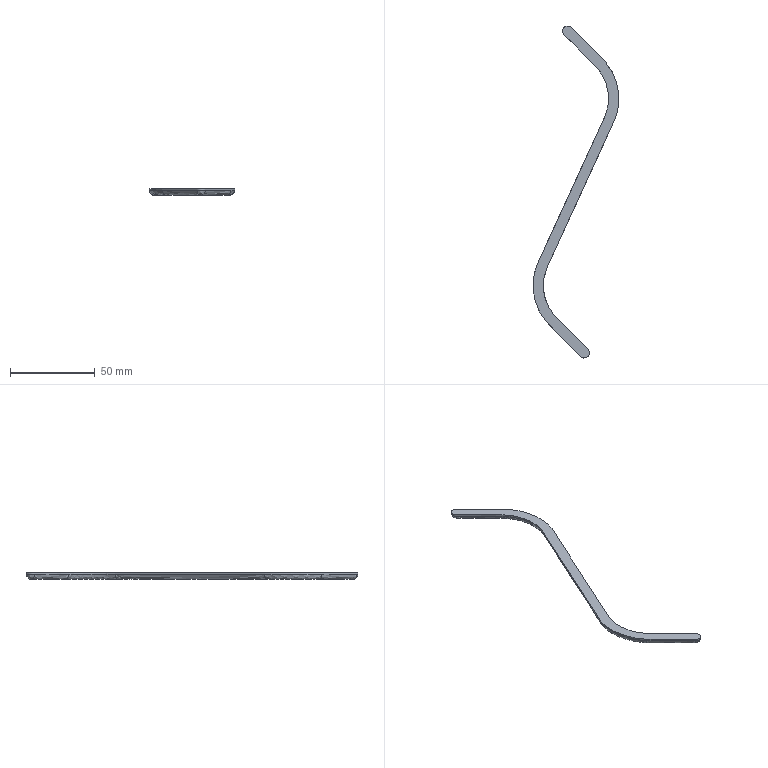Part | STEP file | SL2-MOLD_id526_xmt_txt | 1 solid | 24 faces | box 50.634 x 195.983 x 4 mm | volume 4499 mm3 | other 10 | spline 7 | cylinder 4 | plane 3 | commonest cylinder face diameters 5.8 x4